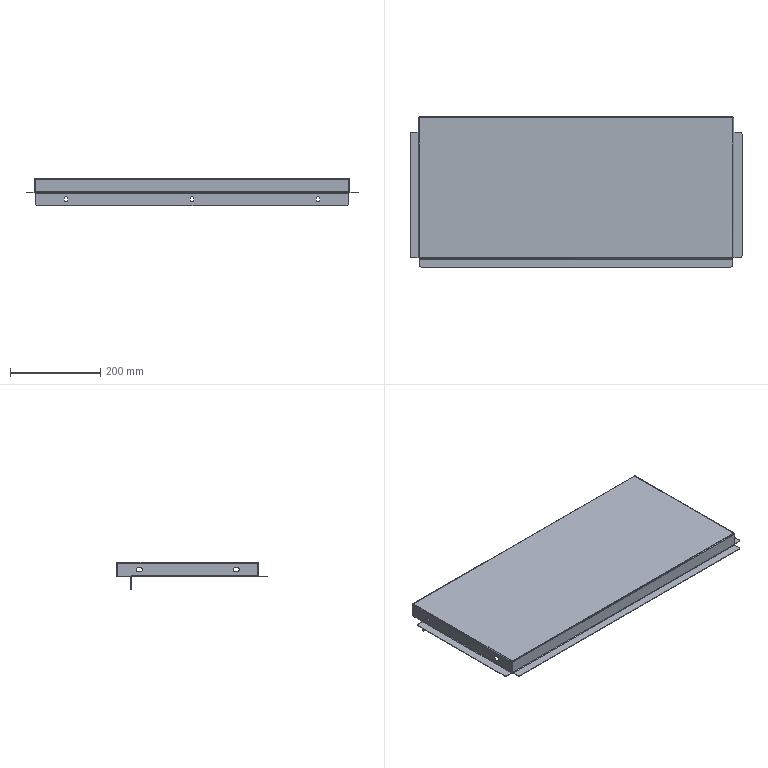Part | SolidWorks | features EdgeFlange 5, ICE 2, Fillet 1, FlatPattern 1, HoleWzd 1, SMBaseFlange 1, SheetMetal 1 | 1 solid | 125 faces | box 737.6 x 333.8 x 60.8 mm | volume 412436 mm3 | plane 74 | cylinder 43 | spline 8 | commonest cylinder face diameters 2 x9 4.4 x9 8 x9 9 x8 10 x8